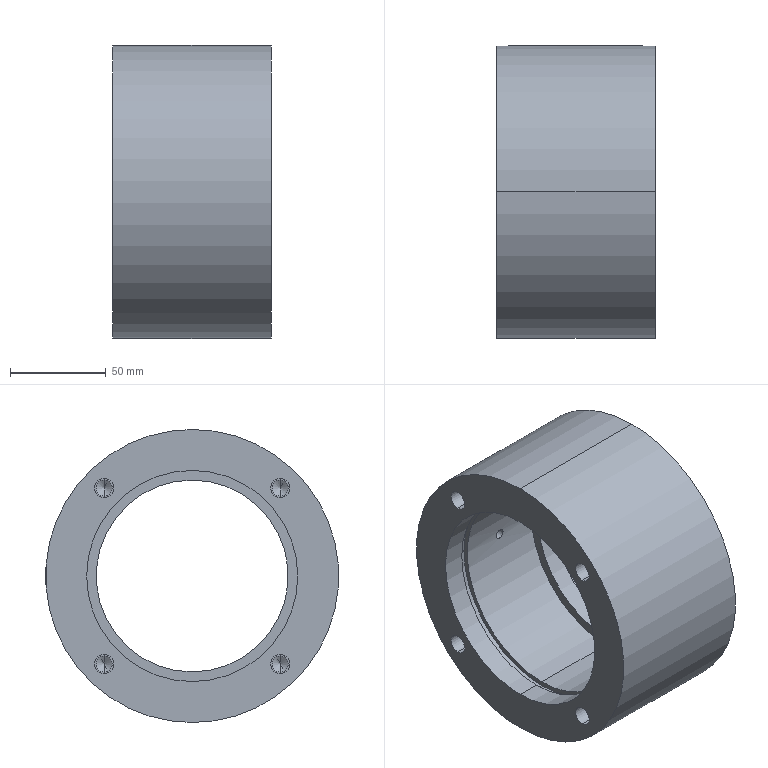Part | STEP file | Input 15 | 1 solid | 51 faces | box 82.5 x 153 x 153 mm | volume 749438 mm3 | cylinder 32 | plane 11 | cone 8 | commonest cylinder face diameters 8.5 x8 10 x8 100.2 x4 110.2 x4 5 x2 104 x2